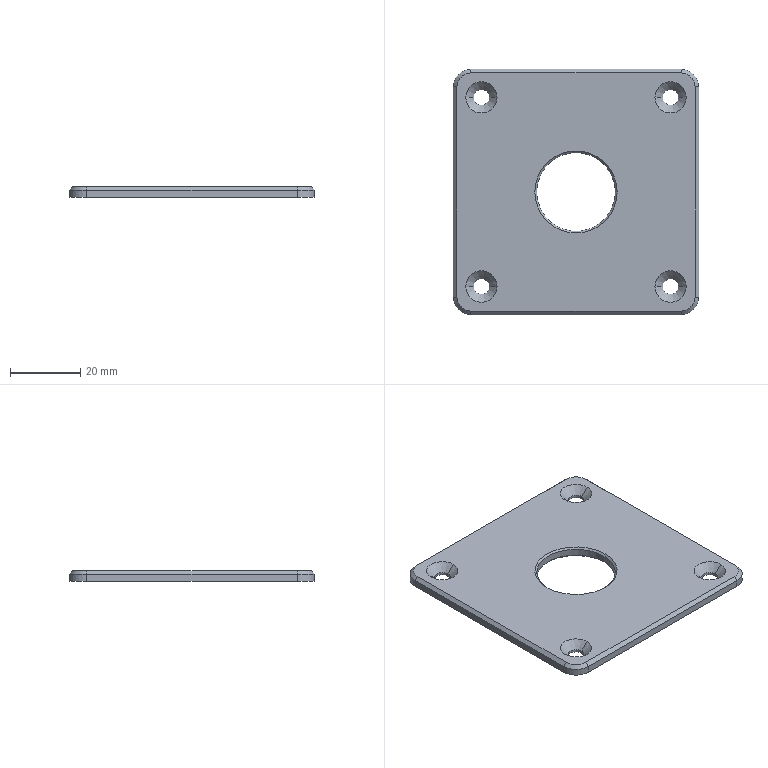Part | STEP file | Push button switch mounting plate 2 | 1 solid | 40 faces | box 70 x 70 x 3 mm | volume 12912 mm3 | cone 16 | cylinder 14 | plane 10 | commonest cylinder face diameters 4.5 x8 10 x4 22.5 x2